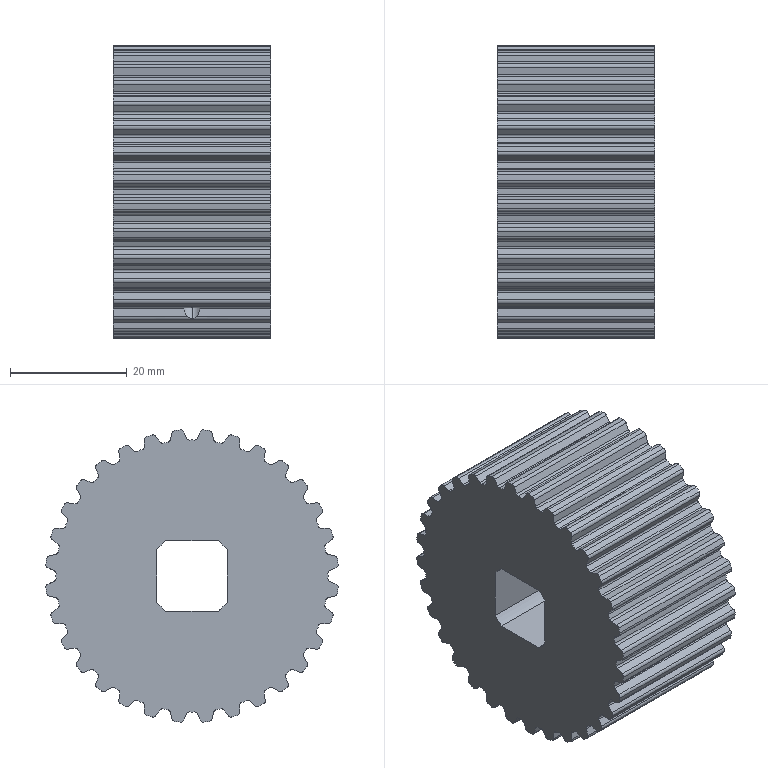Part | STEP file | TTPP32T5250-A-P11_b traction driven pulley | 1 solid | 280 faces | box 27 x 49.946 x 49.946 mm | volume 45519 mm3 | cylinder 206 | plane 74 | commonest cylinder face diameters 0.8 x68 1.2 x64 46.5 x34 50.1 x32 3.242 x4 15 x4